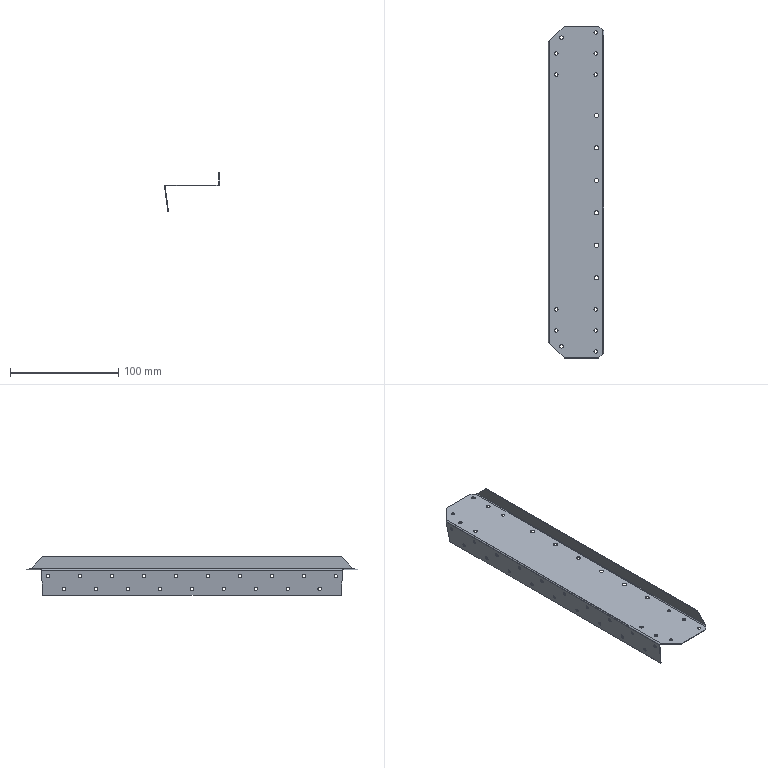Part | SolidWorks | features BaseBody 1 | 1 solid | 102 faces | box 50.86 x 306.6 x 35.812 mm | volume 12373 mm3 | cylinder 78 | plane 18 | spline 6 | commonest cylinder face diameters 3.2 x62 3.855 x12 1.5 x2 2.5 x2